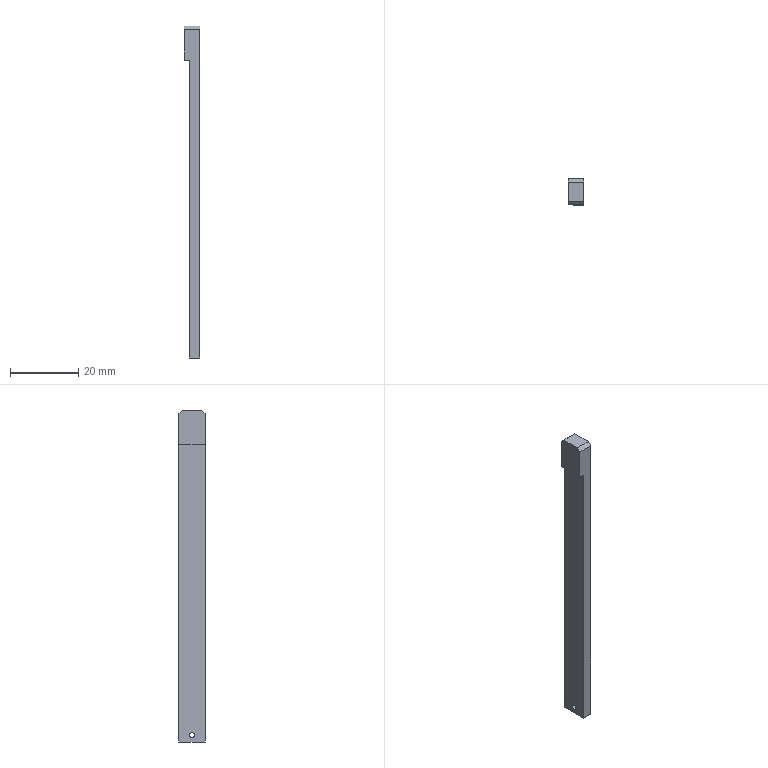Part | STEP file | slingshot detection spring block | 1 solid | 12 faces | box 4.5 x 7.6 x 97 mm | volume 2316 mm3 | plane 10 | cylinder 2 | commonest cylinder face diameters 1.5 x2
STEP:
#1=CARTESIAN_POINT('',(0.,0.,0.));
#2=DIRECTION('',(0.,0.,1.));
#3=DIRECTION('',(1.,0.,0.));
#4=AXIS2_PLACEMENT_3D('',#1,#2,#3);
#5=CARTESIAN_POINT('',(0.,-3.05,28.));
#6=VERTEX_POINT('',#5);
#7=CARTESIAN_POINT('',(3.,-3.05,28.));
#8=VERTEX_POINT('',#7);
#9=CARTESIAN_POINT('',(-22.,-3.05,28.));
#10=DIRECTION('',(1.,0.,0.));
#11=VECTOR('',#10,1.);
#12=LINE('',#9,#11);
#13=CARTESIAN_POINT('',(-22.,-3.8,28.));
#14=DIRECTION('',(1.,0.,0.));
#15=DIRECTION('',(0.,1.,0.));
#16=AXIS2_PLACEMENT_3D('',#13,#14,#15);
#17=CYLINDRICAL_SURFACE('',#16,0.75);
#18=CARTESIAN_POINT('',(6.283,0.));
#19=DIRECTION('',(0.,1.));
#20=VECTOR('',#19,1.);
#21=LINE('',#18,#20);
#22=(GEOMETRIC_REPRESENTATION_CONTEXT(2)PARAMETRIC_REPRESENTATION_CONTEXT()REPRESENTATION_CONTEXT('',''));
#23=DEFINITIONAL_REPRESENTATION('',(#21),#22);
#24=PCURVE('',#17,#23);
#25=CARTESIAN_POINT('',(-22.,-3.8,28.));
#26=DIRECTION('',(1.,0.,0.));
#27=DIRECTION('',(0.,1.,0.));
#28=AXIS2_PLACEMENT_3D('',#25,#26,#27);
#29=CYLINDRICAL_SURFACE('',#28,0.75);
#30=CARTESIAN_POINT('',(0.,0.));
#31=DIRECTION('',(0.,1.));
#32=VECTOR('',#31,1.);
#33=LINE('',#30,#32);
#34=(GEOMETRIC_REPRESENTATION_CONTEXT(2)PARAMETRIC_REPRESENTATION_CONTEXT()REPRESENTATION_CONTEXT('',''));
#35=DEFINITIONAL_REPRESENTATION('',(#33),#34);
#36=PCURVE('',#29,#35);
#37=SURFACE_CURVE('',#12,(#24,#36),.PCURVE_S1.);
#38=EDGE_CURVE('',#6,#8,#37,.T.);
#39=ORIENTED_EDGE('',*,*,#38,.T.);
#40=CARTESIAN_POINT('',(3.,-4.55,28.));
#41=VERTEX_POINT('',#40);
#42=CARTESIAN_POINT('',(3.,-3.8,28.));
#43=DIRECTION('',(1.,0.,0.));
#44=DIRECTION('',(0.,1.,0.));
#45=AXIS2_PLACEMENT_3D('',#42,#43,#44);
#46=CIRCLE('',#45,0.75);
#47=CARTESIAN_POINT('',(0.,25.));
#48=DIRECTION('',(1.,0.));
#49=VECTOR('',#48,1.);
#50=LINE('',#47,#49);
#51=(GEOMETRIC_REPRESENTATION_CONTEXT(2)PARAMETRIC_REPRESENTATION_CONTEXT()REPRESENTATION_CONTEXT('',''));
#52=DEFINITIONAL_REPRESENTATION('',(#50),#51);
#53=PCURVE('',#17,#52);
#54=CARTESIAN_POINT('',(3.,0.,123.));
#55=DIRECTION('',(-1.,0.,0.));
#56=DIRECTION('',(0.,-1.,0.));
#57=AXIS2_PLACEMENT_3D('',#54,#55,#56);
#58=PLANE('',#57);
#59=CARTESIAN_POINT('',(3.05,-95.));
#60=CARTESIAN_POINT('',(3.05,-93.701));
#61=CARTESIAN_POINT('',(4.175,-94.35));
#62=CARTESIAN_POINT('',(5.3,-95.));
#63=CARTESIAN_POINT('',(4.175,-95.65));
#64=CARTESIAN_POINT('',(3.05,-96.299));
#65=CARTESIAN_POINT('',(3.05,-95.));
#66=(BOUNDED_CURVE()B_SPLINE_CURVE(2,(#59,#60,#61,#62,#63,#64,#65),.UNSPECIFIED.,.T.,.F.)B_SPLINE_CURVE_WITH_KNOTS((1,2,2,2,2,1),(-2.094,0.,2.094,4.189,6.283,8.378),.UNSPECIFIED.)CURVE()GEOMETRIC_REPRESENTATION_ITEM()RATIONAL_B_SPLINE_CURVE((1.,0.5,1.,0.5,1.,0.5,1.))REPRESENTATION_ITEM(''));
#67=(GEOMETRIC_REPRESENTATION_CONTEXT(2)PARAMETRIC_REPRESENTATION_CONTEXT()REPRESENTATION_CONTEXT('',''));
#68=DEFINITIONAL_REPRESENTATION('',(#66),#67);
#69=PCURVE('',#58,#68);
#70=SURFACE_CURVE('',#46,(#53,#69),.PCURVE_S1.);
#71=EDGE_CURVE('',#41,#8,#70,.T.);
#72=ORIENTED_EDGE('',*,*,#71,.F.);
#73=CARTESIAN_POINT('',(0.,-4.55,28.));
#74=VERTEX_POINT('',#73);
#75=CARTESIAN_POINT('',(-22.,-4.55,28.));
#76=DIRECTION('',(1.,0.,0.));
#77=VECTOR('',#76,1.);
#78=LINE('',#75,#77);
#79=CARTESIAN_POINT('',(3.142,0.));
#80=DIRECTION('',(0.,1.));
#81=VECTOR('',#80,1.);
#82=LINE('',#79,#81);
#83=(GEOMETRIC_REPRESENTATION_CONTEXT(2)PARAMETRIC_REPRESENTATION_CONTEXT()REPRESENTATION_CONTEXT('',''));
#84=DEFINITIONAL_REPRESENTATION('',(#82),#83);
#85=PCURVE('',#17,#84);
#86=CARTESIAN_POINT('',(3.142,0.));
#87=DIRECTION('',(0.,1.));
#88=VECTOR('',#87,1.);
#89=LINE('',#86,#88);
#90=(GEOMETRIC_REPRESENTATION_CONTEXT(2)PARAMETRIC_REPRESENTATION_CONTEXT()REPRESENTATION_CONTEXT('',''));
#91=DEFINITIONAL_REPRESENTATION('',(#89),#90);
#92=PCURVE('',#29,#91);
#93=SURFACE_CURVE('',#78,(#85,#92),.PCURVE_S1.);
#94=EDGE_CURVE('',#74,#41,#93,.T.);
#95=ORIENTED_EDGE('',*,*,#94,.F.);
#96=CARTESIAN_POINT('',(0.,-3.8,28.));
#97=DIRECTION('',(1.,0.,0.));
#98=DIRECTION('',(0.,1.,0.));
#99=AXIS2_PLACEMENT_3D('',#96,#97,#98);
#100=CIRCLE('',#99,0.75);
#101=CARTESIAN_POINT('',(0.,22.));
#102=DIRECTION('',(1.,0.));
#103=VECTOR('',#102,1.);
#104=LINE('',#101,#103);
#105=(GEOMETRIC_REPRESENTATION_CONTEXT(2)PARAMETRIC_REPRESENTATION_CONTEXT()REPRESENTATION_CONTEXT('',''));
#106=DEFINITIONAL_REPRESENTATION('',(#104),#105);
#107=PCURVE('',#17,#106);
#108=CARTESIAN_POINT('',(0.,0.,123.));
#109=DIRECTION('',(1.,0.,0.));
#110=DIRECTION('',(0.,1.,0.));
#111=AXIS2_PLACEMENT_3D('',#108,#109,#110);
#112=PLANE('',#111);
#113=CARTESIAN_POINT('',(-3.8,-95.));
#114=DIRECTION('',(1.,0.));
#115=AXIS2_PLACEMENT_2D('',#113,#114);
#116=CIRCLE('',#115,0.75);
#117=(GEOMETRIC_REPRESENTATION_CONTEXT(2)PARAMETRIC_REPRESENTATION_CONTEXT()REPRESENTATION_CONTEXT('',''));
#118=DEFINITIONAL_REPRESENTATION('',(#116),#117);
#119=PCURVE('',#112,#118);
#120=SURFACE_CURVE('',#100,(#107,#119),.PCURVE_S1.);
#121=EDGE_CURVE('',#74,#6,#120,.T.);
#122=ORIENTED_EDGE('',*,*,#121,.T.);
#123=EDGE_LOOP('',(#39,#72,#95,#122));
#124=FACE_BOUND('',#123,.F.);
#125=ADVANCED_FACE('',(#124),#17,.F.);
#126=CARTESIAN_POINT('',(0.,-3.8,28.));
#127=DIRECTION('',(1.,0.,0.));
#128=DIRECTION('',(0.,1.,0.));
#129=AXIS2_PLACEMENT_3D('',#126,#127,#128);
#130=CIRCLE('',#129,0.75);
#131=CARTESIAN_POINT('',(-3.8,-95.));
#132=DIRECTION('',(1.,0.));
#133=AXIS2_PLACEMENT_2D('',#131,#132);
#134=CIRCLE('',#133,0.75);
#135=(GEOMETRIC_REPRESENTATION_CONTEXT(2)PARAMETRIC_REPRESENTATION_CONTEXT()REPRESENTATION_CONTEXT('',''));
#136=DEFINITIONAL_REPRESENTATION('',(#134),#135);
#137=PCURVE('',#112,#136);
#138=CARTESIAN_POINT('',(0.,22.));
#139=DIRECTION('',(1.,0.));
#140=VECTOR('',#139,1.);
#141=LINE('',#138,#140);
#142=(GEOMETRIC_REPRESENTATION_CONTEXT(2)PARAMETRIC_REPRESENTATION_CONTEXT()REPRESENTATION_CONTEXT('',''));
#143=DEFINITIONAL_REPRESENTATION('',(#141),#142);
#144=PCURVE('',#29,#143);
#145=SURFACE_CURVE('',#130,(#137,#144),.PCURVE_S1.);
#146=EDGE_CURVE('',#6,#74,#145,.T.);
#147=ORIENTED_EDGE('',*,*,#146,.T.);
#148=ORIENTED_EDGE('',*,*,#121,.T.);
#149=EDGE_LOOP('',(#147,#148));
#150=FACE_BOUND('',#149,.T.);
#151=CARTESIAN_POINT('',(0.,0.,113.));
#152=VERTEX_POINT('',#151);
#153=CARTESIAN_POINT('',(0.,-7.6,113.));
#154=VERTEX_POINT('',#153);
#155=CARTESIAN_POINT('',(0.,0.,113.));
#156=DIRECTION('',(0.,-1.,0.));
#157=VECTOR('',#156,1.);
#158=LINE('',#155,#157);
#159=CARTESIAN_POINT('',(0.,-10.));
#160=DIRECTION('',(-1.,0.));
#161=VECTOR('',#160,1.);
#162=LINE('',#159,#161);
#163=(GEOMETRIC_REPRESENTATION_CONTEXT(2)PARAMETRIC_REPRESENTATION_CONTEXT()REPRESENTATION_CONTEXT('',''));
#164=DEFINITIONAL_REPRESENTATION('',(#162),#163);
#165=PCURVE('',#112,#164);
#166=CARTESIAN_POINT('',(-1.5,0.,113.));
#167=DIRECTION('',(0.,0.,1.));
#168=DIRECTION('',(1.,0.,0.));
#169=AXIS2_PLACEMENT_3D('',#166,#167,#168);
#170=PLANE('',#169);
#171=CARTESIAN_POINT('',(1.5,0.));
#172=DIRECTION('',(0.,-1.));
#173=VECTOR('',#172,1.);
#174=LINE('',#171,#173);
#175=(GEOMETRIC_REPRESENTATION_CONTEXT(2)PARAMETRIC_REPRESENTATION_CONTEXT()REPRESENTATION_CONTEXT('',''));
#176=DEFINITIONAL_REPRESENTATION('',(#174),#175);
#177=PCURVE('',#170,#176);
#178=SURFACE_CURVE('',#158,(#165,#177),.PCURVE_S1.);
#179=EDGE_CURVE('',#152,#154,#178,.T.);
#180=ORIENTED_EDGE('',*,*,#179,.F.);
#181=CARTESIAN_POINT('',(0.,0.,26.));
#182=VERTEX_POINT('',#181);
#183=CARTESIAN_POINT('',(0.,0.,123.));
#184=DIRECTION('',(0.,0.,-1.));
#185=VECTOR('',#184,1.);
#186=LINE('',#183,#185);
#187=CARTESIAN_POINT('',(0.,0.));
#188=DIRECTION('',(0.,-1.));
#189=VECTOR('',#188,1.);
#190=LINE('',#187,#189);
#191=(GEOMETRIC_REPRESENTATION_CONTEXT(2)PARAMETRIC_REPRESENTATION_CONTEXT()REPRESENTATION_CONTEXT('',''));
#192=DEFINITIONAL_REPRESENTATION('',(#190),#191);
#193=PCURVE('',#112,#192);
#194=CARTESIAN_POINT('',(0.,0.,123.));
#195=DIRECTION('',(0.,-1.,0.));
#196=DIRECTION('',(0.,0.,-1.));
#197=AXIS2_PLACEMENT_3D('',#194,#195,#196);
#198=PLANE('',#197);
#199=CARTESIAN_POINT('',(0.,0.));
#200=DIRECTION('',(1.,0.));
#201=VECTOR('',#200,1.);
#202=LINE('',#199,#201);
#203=(GEOMETRIC_REPRESENTATION_CONTEXT(2)PARAMETRIC_REPRESENTATION_CONTEXT()REPRESENTATION_CONTEXT('',''));
#204=DEFINITIONAL_REPRESENTATION('',(#202),#203);
#205=PCURVE('',#198,#204);
#206=SURFACE_CURVE('',#186,(#193,#205),.PCURVE_S1.);
#207=EDGE_CURVE('',#152,#182,#206,.T.);
#208=ORIENTED_EDGE('',*,*,#207,.T.);
#209=CARTESIAN_POINT('',(0.,-7.6,26.));
#210=VERTEX_POINT('',#209);
#211=CARTESIAN_POINT('',(0.,16.05,26.));
#212=DIRECTION('',(0.,1.,0.));
#213=VECTOR('',#212,1.);
#214=LINE('',#211,#213);
#215=CARTESIAN_POINT('',(16.05,-97.));
#216=DIRECTION('',(1.,0.));
#217=VECTOR('',#216,1.);
#218=LINE('',#215,#217);
#219=(GEOMETRIC_REPRESENTATION_CONTEXT(2)PARAMETRIC_REPRESENTATION_CONTEXT()REPRESENTATION_CONTEXT('',''));
#220=DEFINITIONAL_REPRESENTATION('',(#218),#219);
#221=PCURVE('',#112,#220);
#222=CARTESIAN_POINT('',(10.,16.05,26.));
#223=DIRECTION('',(0.,0.,1.));
#224=DIRECTION('',(0.,-1.,0.));
#225=AXIS2_PLACEMENT_3D('',#222,#223,#224);
#226=PLANE('',#225);
#227=CARTESIAN_POINT('',(0.,-10.));
#228=DIRECTION('',(-1.,0.));
#229=VECTOR('',#228,1.);
#230=LINE('',#227,#229);
#231=(GEOMETRIC_REPRESENTATION_CONTEXT(2)PARAMETRIC_REPRESENTATION_CONTEXT()REPRESENTATION_CONTEXT('',''));
#232=DEFINITIONAL_REPRESENTATION('',(#230),#231);
#233=PCURVE('',#226,#232);
#234=SURFACE_CURVE('',#214,(#221,#233),.PCURVE_S1.);
#235=EDGE_CURVE('',#210,#182,#234,.T.);
#236=ORIENTED_EDGE('',*,*,#235,.F.);
#237=CARTESIAN_POINT('',(0.,-7.6,123.));
#238=DIRECTION('',(0.,0.,-1.));
#239=VECTOR('',#238,1.);
#240=LINE('',#237,#239);
#241=CARTESIAN_POINT('',(-7.6,0.));
#242=DIRECTION('',(0.,-1.));
#243=VECTOR('',#242,1.);
#244=LINE('',#241,#243);
#245=(GEOMETRIC_REPRESENTATION_CONTEXT(2)PARAMETRIC_REPRESENTATION_CONTEXT()REPRESENTATION_CONTEXT('',''));
#246=DEFINITIONAL_REPRESENTATION('',(#244),#245);
#247=PCURVE('',#112,#246);
#248=CARTESIAN_POINT('',(0.,-7.6,123.));
#249=DIRECTION('',(0.,1.,0.));
#250=DIRECTION('',(0.,0.,1.));
#251=AXIS2_PLACEMENT_3D('',#248,#249,#250);
#252=PLANE('',#251);
#253=CARTESIAN_POINT('',(0.,0.));
#254=DIRECTION('',(-1.,0.));
#255=VECTOR('',#254,1.);
#256=LINE('',#253,#255);
#257=(GEOMETRIC_REPRESENTATION_CONTEXT(2)PARAMETRIC_REPRESENTATION_CONTEXT()REPRESENTATION_CONTEXT('',''));
#258=DEFINITIONAL_REPRESENTATION('',(#256),#257);
#259=PCURVE('',#252,#258);
#260=SURFACE_CURVE('',#240,(#247,#259),.PCURVE_S1.);
#261=EDGE_CURVE('',#154,#210,#260,.T.);
#262=ORIENTED_EDGE('',*,*,#261,.F.);
#263=EDGE_LOOP('',(#180,#208,#236,#262));
#264=FACE_BOUND('',#263,.T.);
#265=ADVANCED_FACE('',(#150,#264),#112,.F.);
#266=CARTESIAN_POINT('',(3.,-7.6,122.));
#267=VERTEX_POINT('',#266);
#268=CARTESIAN_POINT('',(-1.5,-7.6,122.));
#269=VERTEX_POINT('',#268);
#270=CARTESIAN_POINT('',(0.,-7.6,122.));
#271=DIRECTION('',(-1.,0.,0.));
#272=VECTOR('',#271,1.);
#273=LINE('',#270,#272);
#274=CARTESIAN_POINT('',(-1.,0.));
#275=DIRECTION('',(0.,-1.));
#276=VECTOR('',#275,1.);
#277=LINE('',#274,#276);
#278=(GEOMETRIC_REPRESENTATION_CONTEXT(2)PARAMETRIC_REPRESENTATION_CONTEXT()REPRESENTATION_CONTEXT('',''));
#279=DEFINITIONAL_REPRESENTATION('',(#277),#278);
#280=PCURVE('',#252,#279);
#281=CARTESIAN_POINT('',(0.,-6.6,123.));
#282=DIRECTION('',(0.,-0.7071,0.7071));
#283=DIRECTION('',(0.,-0.7071,-0.7071));
#284=AXIS2_PLACEMENT_3D('',#281,#282,#283);
#285=PLANE('',#284);
#286=CARTESIAN_POINT('',(1.414,0.));
#287=DIRECTION('',(0.,-1.));
#288=VECTOR('',#287,1.);
#289=LINE('',#286,#288);
#290=(GEOMETRIC_REPRESENTATION_CONTEXT(2)PARAMETRIC_REPRESENTATION_CONTEXT()REPRESENTATION_CONTEXT('',''));
#291=DEFINITIONAL_REPRESENTATION('',(#289),#290);
#292=PCURVE('',#285,#291);
#293=SURFACE_CURVE('',#273,(#280,#292),.PCURVE_S1.);
#294=EDGE_CURVE('',#267,#269,#293,.T.);
#295=ORIENTED_EDGE('',*,*,#294,.T.);
#296=CARTESIAN_POINT('',(-1.5,-7.6,113.));
#297=VERTEX_POINT('',#296);
#298=CARTESIAN_POINT('',(-1.5,-7.6,113.));
#299=DIRECTION('',(0.,0.,1.));
#300=VECTOR('',#299,1.);
#301=LINE('',#298,#300);
#302=CARTESIAN_POINT('',(-10.,-1.5));
#303=DIRECTION('',(1.,0.));
#304=VECTOR('',#303,1.);
#305=LINE('',#302,#304);
#306=(GEOMETRIC_REPRESENTATION_CONTEXT(2)PARAMETRIC_REPRESENTATION_CONTEXT()REPRESENTATION_CONTEXT('',''));
#307=DEFINITIONAL_REPRESENTATION('',(#305),#306);
#308=PCURVE('',#252,#307);
#309=CARTESIAN_POINT('',(-1.5,-3.8,125.8));
#310=DIRECTION('',(1.,0.,0.));
#311=DIRECTION('',(0.,1.,0.));
#312=AXIS2_PLACEMENT_3D('',#309,#310,#311);
#313=PLANE('',#312);
#314=CARTESIAN_POINT('',(-3.8,-12.8));
#315=DIRECTION('',(0.,1.));
#316=VECTOR('',#315,1.);
#317=LINE('',#314,#316);
#318=(GEOMETRIC_REPRESENTATION_CONTEXT(2)PARAMETRIC_REPRESENTATION_CONTEXT()REPRESENTATION_CONTEXT('',''));
#319=DEFINITIONAL_REPRESENTATION('',(#317),#318);
#320=PCURVE('',#313,#319);
#321=SURFACE_CURVE('',#301,(#308,#320),.PCURVE_S1.);
#322=EDGE_CURVE('',#297,#269,#321,.T.);
#323=ORIENTED_EDGE('',*,*,#322,.F.);
#324=CARTESIAN_POINT('',(-1.5,-7.6,113.));
#325=DIRECTION('',(1.,0.,0.));
#326=VECTOR('',#325,1.);
#327=LINE('',#324,#326);
#328=CARTESIAN_POINT('',(-10.,-1.5));
#329=DIRECTION('',(0.,1.));
#330=VECTOR('',#329,1.);
#331=LINE('',#328,#330);
#332=(GEOMETRIC_REPRESENTATION_CONTEXT(2)PARAMETRIC_REPRESENTATION_CONTEXT()REPRESENTATION_CONTEXT('',''));
#333=DEFINITIONAL_REPRESENTATION('',(#331),#332);
#334=PCURVE('',#252,#333);
#335=CARTESIAN_POINT('',(0.,-7.6));
#336=DIRECTION('',(1.,0.));
#337=VECTOR('',#336,1.);
#338=LINE('',#335,#337);
#339=(GEOMETRIC_REPRESENTATION_CONTEXT(2)PARAMETRIC_REPRESENTATION_CONTEXT()REPRESENTATION_CONTEXT('',''));
#340=DEFINITIONAL_REPRESENTATION('',(#338),#339);
#341=PCURVE('',#170,#340);
#342=SURFACE_CURVE('',#327,(#334,#341),.PCURVE_S1.);
#343=EDGE_CURVE('',#297,#154,#342,.T.);
#344=ORIENTED_EDGE('',*,*,#343,.T.);
#345=ORIENTED_EDGE('',*,*,#261,.T.);
#346=CARTESIAN_POINT('',(3.,-7.6,26.));
#347=VERTEX_POINT('',#346);
#348=CARTESIAN_POINT('',(0.,-7.6,26.));
#349=DIRECTION('',(1.,0.,0.));
#350=VECTOR('',#349,1.);
#351=LINE('',#348,#350);
#352=CARTESIAN_POINT('',(-97.,0.));
#353=DIRECTION('',(0.,1.));
#354=VECTOR('',#353,1.);
#355=LINE('',#352,#354);
#356=(GEOMETRIC_REPRESENTATION_CONTEXT(2)PARAMETRIC_REPRESENTATION_CONTEXT()REPRESENTATION_CONTEXT('',''));
#357=DEFINITIONAL_REPRESENTATION('',(#355),#356);
#358=PCURVE('',#252,#357);
#359=CARTESIAN_POINT('',(23.65,-10.));
#360=DIRECTION('',(0.,1.));
#361=VECTOR('',#360,1.);
#362=LINE('',#359,#361);
#363=(GEOMETRIC_REPRESENTATION_CONTEXT(2)PARAMETRIC_REPRESENTATION_CONTEXT()REPRESENTATION_CONTEXT('',''));
#364=DEFINITIONAL_REPRESENTATION('',(#362),#363);
#365=PCURVE('',#226,#364);
#366=SURFACE_CURVE('',#351,(#358,#365),.PCURVE_S1.);
#367=EDGE_CURVE('',#210,#347,#366,.T.);
#368=ORIENTED_EDGE('',*,*,#367,.T.);
#369=CARTESIAN_POINT('',(3.,-7.6,123.));
#370=DIRECTION('',(0.,0.,-1.));
#371=VECTOR('',#370,1.);
#372=LINE('',#369,#371);
#373=CARTESIAN_POINT('',(0.,3.));
#374=DIRECTION('',(-1.,0.));
#375=VECTOR('',#374,1.);
#376=LINE('',#373,#375);
#377=(GEOMETRIC_REPRESENTATION_CONTEXT(2)PARAMETRIC_REPRESENTATION_CONTEXT()REPRESENTATION_CONTEXT('',''));
#378=DEFINITIONAL_REPRESENTATION('',(#376),#377);
#379=PCURVE('',#252,#378);
#380=CARTESIAN_POINT('',(7.6,0.));
#381=DIRECTION('',(0.,-1.));
#382=VECTOR('',#381,1.);
#383=LINE('',#380,#382);
#384=(GEOMETRIC_REPRESENTATION_CONTEXT(2)PARAMETRIC_REPRESENTATION_CONTEXT()REPRESENTATION_CONTEXT('',''));
#385=DEFINITIONAL_REPRESENTATION('',(#383),#384);
#386=PCURVE('',#58,#385);
#387=SURFACE_CURVE('',#372,(#379,#386),.PCURVE_S1.);
#388=EDGE_CURVE('',#267,#347,#387,.T.);
#389=ORIENTED_EDGE('',*,*,#388,.F.);
#390=EDGE_LOOP('',(#295,#323,#344,#345,#368,#389));
#391=FACE_BOUND('',#390,.T.);
#392=ADVANCED_FACE('',(#391),#252,.F.);
#393=CARTESIAN_POINT('',(3.,-3.8,28.));
#394=DIRECTION('',(1.,0.,0.));
#395=DIRECTION('',(0.,1.,0.));
#396=AXIS2_PLACEMENT_3D('',#393,#394,#395);
#397=CIRCLE('',#396,0.75);
#398=CARTESIAN_POINT('',(3.05,-95.));
#399=CARTESIAN_POINT('',(3.05,-93.701));
#400=CARTESIAN_POINT('',(4.175,-94.35));
#401=CARTESIAN_POINT('',(5.3,-95.));
#402=CARTESIAN_POINT('',(4.175,-95.65));
#403=CARTESIAN_POINT('',(3.05,-96.299));
#404=CARTESIAN_POINT('',(3.05,-95.));
#405=(BOUNDED_CURVE()B_SPLINE_CURVE(2,(#398,#399,#400,#401,#402,#403,#404),.UNSPECIFIED.,.T.,.F.)B_SPLINE_CURVE_WITH_KNOTS((1,2,2,2,2,1),(-2.094,0.,2.094,4.189,6.283,8.378),.UNSPECIFIED.)CURVE()GEOMETRIC_REPRESENTATION_ITEM()RATIONAL_B_SPLINE_CURVE((1.,0.5,1.,0.5,1.,0.5,1.))REPRESENTATION_ITEM(''));
#406=(GEOMETRIC_REPRESENTATION_CONTEXT(2)PARAMETRIC_REPRESENTATION_CONTEXT()REPRESENTATION_CONTEXT('',''));
#407=DEFINITIONAL_REPRESENTATION('',(#405),#406);
#408=PCURVE('',#58,#407);
#409=CARTESIAN_POINT('',(0.,25.));
#410=DIRECTION('',(1.,0.));
#411=VECTOR('',#410,1.);
#412=LINE('',#409,#411);
#413=(GEOMETRIC_REPRESENTATION_CONTEXT(2)PARAMETRIC_REPRESENTATION_CONTEXT()REPRESENTATION_CONTEXT('',''));
#414=DEFINITIONAL_REPRESENTATION('',(#412),#413);
#415=PCURVE('',#29,#414);
#416=SURFACE_CURVE('',#397,(#408,#415),.PCURVE_S1.);
#417=EDGE_CURVE('',#8,#41,#416,.T.);
#418=ORIENTED_EDGE('',*,*,#417,.F.);
#419=ORIENTED_EDGE('',*,*,#71,.F.);
#420=EDGE_LOOP('',(#418,#419));
#421=FACE_BOUND('',#420,.T.);
#422=ORIENTED_EDGE('',*,*,#388,.T.);
#423=CARTESIAN_POINT('',(3.,0.,26.));
#424=VERTEX_POINT('',#423);
#425=CARTESIAN_POINT('',(3.,0.,26.));
#426=DIRECTION('',(0.,1.,0.));
#427=VECTOR('',#426,1.);
#428=LINE('',#425,#427);
#429=CARTESIAN_POINT('',(0.,-97.));
#430=DIRECTION('',(-1.,0.));
#431=VECTOR('',#430,1.);
#432=LINE('',#429,#431);
#433=(GEOMETRIC_REPRESENTATION_CONTEXT(2)PARAMETRIC_REPRESENTATION_CONTEXT()REPRESENTATION_CONTEXT('',''));
#434=DEFINITIONAL_REPRESENTATION('',(#432),#433);
#435=PCURVE('',#58,#434);
#436=CARTESIAN_POINT('',(16.05,-7.));
#437=DIRECTION('',(-1.,0.));
#438=VECTOR('',#437,1.);
#439=LINE('',#436,#438);
#440=(GEOMETRIC_REPRESENTATION_CONTEXT(2)PARAMETRIC_REPRESENTATION_CONTEXT()REPRESENTATION_CONTEXT('',''));
#441=DEFINITIONAL_REPRESENTATION('',(#439),#440);
#442=PCURVE('',#226,#441);
#443=SURFACE_CURVE('',#428,(#435,#442),.PCURVE_S1.);
#444=EDGE_CURVE('',#347,#424,#443,.T.);
#445=ORIENTED_EDGE('',*,*,#444,.T.);
#446=CARTESIAN_POINT('',(3.,0.,122.));
#447=VERTEX_POINT('',#446);
#448=CARTESIAN_POINT('',(3.,0.,123.));
#449=DIRECTION('',(0.,0.,-1.));
#450=VECTOR('',#449,1.);
#451=LINE('',#448,#450);
#452=CARTESIAN_POINT('',(0.,0.));
#453=DIRECTION('',(0.,-1.));
#454=VECTOR('',#453,1.);
#455=LINE('',#452,#454);
#456=(GEOMETRIC_REPRESENTATION_CONTEXT(2)PARAMETRIC_REPRESENTATION_CONTEXT()REPRESENTATION_CONTEXT('',''));
#457=DEFINITIONAL_REPRESENTATION('',(#455),#456);
#458=PCURVE('',#58,#457);
#459=CARTESIAN_POINT('',(0.,3.));
#460=DIRECTION('',(1.,0.));
#461=VECTOR('',#460,1.);
#462=LINE('',#459,#461);
#463=(GEOMETRIC_REPRESENTATION_CONTEXT(2)PARAMETRIC_REPRESENTATION_CONTEXT()REPRESENTATION_CONTEXT('',''));
#464=DEFINITIONAL_REPRESENTATION('',(#462),#463);
#465=PCURVE('',#198,#464);
#466=SURFACE_CURVE('',#451,(#458,#465),.PCURVE_S1.);
#467=EDGE_CURVE('',#447,#424,#466,.T.);
#468=ORIENTED_EDGE('',*,*,#467,.F.);
#469=CARTESIAN_POINT('',(3.,-1.,123.));
#470=VERTEX_POINT('',#469);
#471=CARTESIAN_POINT('',(3.,-1.,123.));
#472=DIRECTION('',(0.,-0.7071,0.7071));
#473=VECTOR('',#472,1.);
#474=LINE('',#471,#473);
#475=CARTESIAN_POINT('',(1.,0.));
#476=DIRECTION('',(0.7071,0.7071));
#477=VECTOR('',#476,1.);
#478=LINE('',#475,#477);
#479=(GEOMETRIC_REPRESENTATION_CONTEXT(2)PARAMETRIC_REPRESENTATION_CONTEXT()REPRESENTATION_CONTEXT('',''));
#480=DEFINITIONAL_REPRESENTATION('',(#478),#479);
#481=PCURVE('',#58,#480);
#482=CARTESIAN_POINT('',(0.,-1.,123.));
#483=DIRECTION('',(0.,0.7071,0.7071));
#484=DIRECTION('',(0.,-0.7071,0.7071));
#485=AXIS2_PLACEMENT_3D('',#482,#483,#484);
#486=PLANE('',#485);
#487=CARTESIAN_POINT('',(0.,3.));
#488=DIRECTION('',(1.,0.));
#489=VECTOR('',#488,1.);
#490=LINE('',#487,#489);
#491=(GEOMETRIC_REPRESENTATION_CONTEXT(2)PARAMETRIC_REPRESENTATION_CONTEXT()REPRESENTATION_CONTEXT('',''));
#492=DEFINITIONAL_REPRESENTATION('',(#490),#491);
#493=PCURVE('',#486,#492);
#494=SURFACE_CURVE('',#474,(#481,#493),.PCURVE_S1.);
#495=EDGE_CURVE('',#447,#470,#494,.T.);
#496=ORIENTED_EDGE('',*,*,#495,.T.);
#497=CARTESIAN_POINT('',(3.,-6.6,123.));
#498=VERTEX_POINT('',#497);
#499=CARTESIAN_POINT('',(3.,0.,123.));
#500=DIRECTION('',(0.,1.,0.));
#501=VECTOR('',#500,1.);
#502=LINE('',#499,#501);
#503=CARTESIAN_POINT('',(0.,0.));
#504=DIRECTION('',(-1.,0.));
#505=VECTOR('',#504,1.);
#506=LINE('',#503,#505);
#507=(GEOMETRIC_REPRESENTATION_CONTEXT(2)PARAMETRIC_REPRESENTATION_CONTEXT()REPRESENTATION_CONTEXT('',''));
#508=DEFINITIONAL_REPRESENTATION('',(#506),#507);
#509=PCURVE('',#58,#508);
#510=CARTESIAN_POINT('',(0.,-7.6,123.));
#511=DIRECTION('',(0.,0.,1.));
#512=DIRECTION('',(1.,0.,0.));
#513=AXIS2_PLACEMENT_3D('',#510,#511,#512);
#514=PLANE('',#513);
#515=CARTESIAN_POINT('',(3.,7.6));
#516=DIRECTION('',(0.,1.));
#517=VECTOR('',#516,1.);
#518=LINE('',#515,#517);
#519=(GEOMETRIC_REPRESENTATION_CONTEXT(2)PARAMETRIC_REPRESENTATION_CONTEXT()REPRESENTATION_CONTEXT('',''));
#520=DEFINITIONAL_REPRESENTATION('',(#518),#519);
#521=PCURVE('',#514,#520);
#522=SURFACE_CURVE('',#502,(#509,#521),.PCURVE_S1.);
#523=EDGE_CURVE('',#498,#470,#522,.T.);
#524=ORIENTED_EDGE('',*,*,#523,.F.);
#525=CARTESIAN_POINT('',(3.,-6.6,123.));
#526=DIRECTION('',(0.,-0.7071,-0.7071));
#527=VECTOR('',#526,1.);
#528=LINE('',#525,#527);
#529=CARTESIAN_POINT('',(6.6,0.));
#530=DIRECTION('',(0.7071,-0.7071));
#531=VECTOR('',#530,1.);
#532=LINE('',#529,#531);
#533=(GEOMETRIC_REPRESENTATION_CONTEXT(2)PARAMETRIC_REPRESENTATION_CONTEXT()REPRESENTATION_CONTEXT('',''));
#534=DEFINITIONAL_REPRESENTATION('',(#532),#533);
#535=PCURVE('',#58,#534);
#536=CARTESIAN_POINT('',(0.,3.));
#537=DIRECTION('',(1.,0.));
#538=VECTOR('',#537,1.);
#539=LINE('',#536,#538);
#540=(GEOMETRIC_REPRESENTATION_CONTEXT(2)PARAMETRIC_REPRESENTATION_CONTEXT()REPRESENTATION_CONTEXT('',''));
#541=DEFINITIONAL_REPRESENTATION('',(#539),#540);
#542=PCURVE('',#285,#541);
#543=SURFACE_CURVE('',#528,(#535,#542),.PCURVE_S1.);
#544=EDGE_CURVE('',#498,#267,#543,.T.);
#545=ORIENTED_EDGE('',*,*,#544,.T.);
#546=EDGE_LOOP('',(#422,#445,#468,#496,#524,#545));
#547=FACE_BOUND('',#546,.T.);
#548=ADVANCED_FACE('',(#421,#547),#58,.F.);
#549=ORIENTED_EDGE('',*,*,#467,.T.);
#550=CARTESIAN_POINT('',(0.,0.,26.));
#551=DIRECTION('',(-1.,0.,0.));
#552=VECTOR('',#551,1.);
#553=LINE('',#550,#552);
#554=CARTESIAN_POINT('',(97.,0.));
#555=DIRECTION('',(0.,-1.));
#556=VECTOR('',#555,1.);
#557=LINE('',#554,#556);
#558=(GEOMETRIC_REPRESENTATION_CONTEXT(2)PARAMETRIC_REPRESENTATION_CONTEXT()REPRESENTATION_CONTEXT('',''));
#559=DEFINITIONAL_REPRESENTATION('',(#557),#558);
#560=PCURVE('',#198,#559);
#561=CARTESIAN_POINT('',(16.05,-10.));
#562=DIRECTION('',(0.,-1.));
#563=VECTOR('',#562,1.);
#564=LINE('',#561,#563);
#565=(GEOMETRIC_REPRESENTATION_CONTEXT(2)PARAMETRIC_REPRESENTATION_CONTEXT()REPRESENTATION_CONTEXT('',''));
#566=DEFINITIONAL_REPRESENTATION('',(#564),#565);
#567=PCURVE('',#226,#566);
#568=SURFACE_CURVE('',#553,(#560,#567),.PCURVE_S1.);
#569=EDGE_CURVE('',#424,#182,#568,.T.);
#570=ORIENTED_EDGE('',*,*,#569,.T.);
#571=ORIENTED_EDGE('',*,*,#207,.F.);
#572=CARTESIAN_POINT('',(-1.5,0.,113.));
#573=VERTEX_POINT('',#572);
#574=CARTESIAN_POINT('',(-1.5,0.,113.));
#575=DIRECTION('',(1.,0.,0.));
#576=VECTOR('',#575,1.);
#577=LINE('',#574,#576);
#578=CARTESIAN_POINT('',(10.,-1.5));
#579=DIRECTION('',(0.,1.));
#580=VECTOR('',#579,1.);
#581=LINE('',#578,#580);
#582=(GEOMETRIC_REPRESENTATION_CONTEXT(2)PARAMETRIC_REPRESENTATION_CONTEXT()REPRESENTATION_CONTEXT('',''));
#583=DEFINITIONAL_REPRESENTATION('',(#581),#582);
#584=PCURVE('',#198,#583);
#585=CARTESIAN_POINT('',(0.,0.));
#586=DIRECTION('',(1.,0.));
#587=VECTOR('',#586,1.);
#588=LINE('',#585,#587);
#589=(GEOMETRIC_REPRESENTATION_CONTEXT(2)PARAMETRIC_REPRESENTATION_CONTEXT()REPRESENTATION_CONTEXT('',''));
#590=DEFINITIONAL_REPRESENTATION('',(#588),#589);
#591=PCURVE('',#170,#590);
#592=SURFACE_CURVE('',#577,(#584,#591),.PCURVE_S1.);
#593=EDGE_CURVE('',#573,#152,#592,.T.);
#594=ORIENTED_EDGE('',*,*,#593,.F.);
#595=CARTESIAN_POINT('',(-1.5,0.,122.));
#596=VERTEX_POINT('',#595);
#597=CARTESIAN_POINT('',(-1.5,0.,122.));
#598=DIRECTION('',(0.,0.,-1.));
#599=VECTOR('',#598,1.);
#600=LINE('',#597,#599);
#601=CARTESIAN_POINT('',(1.,-1.5));
#602=DIRECTION('',(1.,0.));
#603=VECTOR('',#602,1.);
#604=LINE('',#601,#603);
#605=(GEOMETRIC_REPRESENTATION_CONTEXT(2)PARAMETRIC_REPRESENTATION_CONTEXT()REPRESENTATION_CONTEXT('',''));
#606=DEFINITIONAL_REPRESENTATION('',(#604),#605);
#607=PCURVE('',#198,#606);
#608=CARTESIAN_POINT('',(3.8,-3.8));
#609=DIRECTION('',(0.,-1.));
#610=VECTOR('',#609,1.);
#611=LINE('',#608,#610);
#612=(GEOMETRIC_REPRESENTATION_CONTEXT(2)PARAMETRIC_REPRESENTATION_CONTEXT()REPRESENTATION_CONTEXT('',''));
#613=DEFINITIONAL_REPRESENTATION('',(#611),#612);
#614=PCURVE('',#313,#613);
#615=SURFACE_CURVE('',#600,(#607,#614),.PCURVE_S1.);
#616=EDGE_CURVE('',#596,#573,#615,.T.);
#617=ORIENTED_EDGE('',*,*,#616,.F.);
#618=CARTESIAN_POINT('',(3.,0.,122.));
#619=DIRECTION('',(1.,0.,0.));
#620=VECTOR('',#619,1.);
#621=LINE('',#618,#620);
#622=CARTESIAN_POINT('',(1.,3.));
#623=DIRECTION('',(0.,1.));
#624=VECTOR('',#623,1.);
#625=LINE('',#622,#624);
#626=(GEOMETRIC_REPRESENTATION_CONTEXT(2)PARAMETRIC_REPRESENTATION_CONTEXT()REPRESENTATION_CONTEXT('',''));
#627=DEFINITIONAL_REPRESENTATION('',(#625),#626);
#628=PCURVE('',#198,#627);
#629=CARTESIAN_POINT('',(-1.414,3.));
#630=DIRECTION('',(0.,1.));
#631=VECTOR('',#630,1.);
#632=LINE('',#629,#631);
#633=(GEOMETRIC_REPRESENTATION_CONTEXT(2)PARAMETRIC_REPRESENTATION_CONTEXT()REPRESENTATION_CONTEXT('',''));
#634=DEFINITIONAL_REPRESENTATION('',(#632),#633);
#635=PCURVE('',#486,#634);
#636=SURFACE_CURVE('',#621,(#628,#635),.PCURVE_S1.);
#637=EDGE_CURVE('',#596,#447,#636,.T.);
#638=ORIENTED_EDGE('',*,*,#637,.T.);
#639=EDGE_LOOP('',(#549,#570,#571,#594,#617,#638));
#640=FACE_BOUND('',#639,.T.);
#641=ADVANCED_FACE('',(#640),#198,.F.);
#642=ORIENTED_EDGE('',*,*,#523,.T.);
#643=CARTESIAN_POINT('',(-1.5,-1.,123.));
#644=VERTEX_POINT('',#643);
#645=CARTESIAN_POINT('',(0.,-1.,123.));
#646=DIRECTION('',(-1.,0.,0.));
#647=VECTOR('',#646,1.);
#648=LINE('',#645,#647);
#649=CARTESIAN_POINT('',(0.,6.6));
#650=DIRECTION('',(-1.,0.));
#651=VECTOR('',#650,1.);
#652=LINE('',#649,#651);
#653=(GEOMETRIC_REPRESENTATION_CONTEXT(2)PARAMETRIC_REPRESENTATION_CONTEXT()REPRESENTATION_CONTEXT('',''));
#654=DEFINITIONAL_REPRESENTATION('',(#652),#653);
#655=PCURVE('',#514,#654);
#656=CARTESIAN_POINT('',(0.,0.));
#657=DIRECTION('',(0.,-1.));
#658=VECTOR('',#657,1.);
#659=LINE('',#656,#658);
#660=(GEOMETRIC_REPRESENTATION_CONTEXT(2)PARAMETRIC_REPRESENTATION_CONTEXT()REPRESENTATION_CONTEXT('',''));
#661=DEFINITIONAL_REPRESENTATION('',(#659),#660);
#662=PCURVE('',#486,#661);
#663=SURFACE_CURVE('',#648,(#655,#662),.PCURVE_S1.);
#664=EDGE_CURVE('',#470,#644,#663,.T.);
#665=ORIENTED_EDGE('',*,*,#664,.T.);
#666=CARTESIAN_POINT('',(-1.5,-6.6,123.));
#667=VERTEX_POINT('',#666);
#668=CARTESIAN_POINT('',(-1.5,-6.6,123.));
#669=DIRECTION('',(0.,1.,0.));
#670=VECTOR('',#669,1.);
#671=LINE('',#668,#670);
#672=CARTESIAN_POINT('',(-1.5,1.));
#673=DIRECTION('',(0.,1.));
#674=VECTOR('',#673,1.);
#675=LINE('',#672,#674);
#676=(GEOMETRIC_REPRESENTATION_CONTEXT(2)PARAMETRIC_REPRESENTATION_CONTEXT()REPRESENTATION_CONTEXT('',''));
#677=DEFINITIONAL_REPRESENTATION('',(#675),#676);
#678=PCURVE('',#514,#677);
#679=CARTESIAN_POINT('',(-2.8,-2.8));
#680=DIRECTION('',(1.,0.));
#681=VECTOR('',#680,1.);
#682=LINE('',#679,#681);
#683=(GEOMETRIC_REPRESENTATION_CONTEXT(2)PARAMETRIC_REPRESENTATION_CONTEXT()REPRESENTATION_CONTEXT('',''));
#684=DEFINITIONAL_REPRESENTATION('',(#682),#683);
#685=PCURVE('',#313,#684);
#686=SURFACE_CURVE('',#671,(#678,#685),.PCURVE_S1.);
#687=EDGE_CURVE('',#667,#644,#686,.T.);
#688=ORIENTED_EDGE('',*,*,#687,.F.);
#689=CARTESIAN_POINT('',(3.,-6.6,123.));
#690=DIRECTION('',(1.,0.,0.));
#691=VECTOR('',#690,1.);
#692=LINE('',#689,#691);
#693=CARTESIAN_POINT('',(3.,1.));
#694=DIRECTION('',(1.,0.));
#695=VECTOR('',#694,1.);
#696=LINE('',#693,#695);
#697=(GEOMETRIC_REPRESENTATION_CONTEXT(2)PARAMETRIC_REPRESENTATION_CONTEXT()REPRESENTATION_CONTEXT('',''));
#698=DEFINITIONAL_REPRESENTATION('',(#696),#697);
#699=PCURVE('',#514,#698);
#700=CARTESIAN_POINT('',(0.,3.));
#701=DIRECTION('',(0.,1.));
#702=VECTOR('',#701,1.);
#703=LINE('',#700,#702);
#704=(GEOMETRIC_REPRESENTATION_CONTEXT(2)PARAMETRIC_REPRESENTATION_CONTEXT()REPRESENTATION_CONTEXT('',''));
#705=DEFINITIONAL_REPRESENTATION('',(#703),#704);
#706=PCURVE('',#285,#705);
#707=SURFACE_CURVE('',#692,(#699,#706),.PCURVE_S1.);
#708=EDGE_CURVE('',#667,#498,#707,.T.);
#709=ORIENTED_EDGE('',*,*,#708,.T.);
#710=EDGE_LOOP('',(#642,#665,#688,#709));
#711=FACE_BOUND('',#710,.T.);
#712=ADVANCED_FACE('',(#711),#514,.T.);
#713=ORIENTED_EDGE('',*,*,#495,.F.);
#714=ORIENTED_EDGE('',*,*,#637,.F.);
#715=CARTESIAN_POINT('',(-1.5,-1.,123.));
#716=DIRECTION('',(0.,0.7071,-0.7071));
#717=VECTOR('',#716,1.);
#718=LINE('',#715,#717);
#719=CARTESIAN_POINT('',(0.,-1.5));
#720=DIRECTION('',(-1.,0.));
#721=VECTOR('',#720,1.);
#722=LINE('',#719,#721);
#723=(GEOMETRIC_REPRESENTATION_CONTEXT(2)PARAMETRIC_REPRESENTATION_CONTEXT()REPRESENTATION_CONTEXT('',''));
#724=DEFINITIONAL_REPRESENTATION('',(#722),#723);
#725=PCURVE('',#486,#724);
#726=CARTESIAN_POINT('',(2.8,-2.8));
#727=DIRECTION('',(0.7071,-0.7071));
#728=VECTOR('',#727,1.);
#729=LINE('',#726,#728);
#730=(GEOMETRIC_REPRESENTATION_CONTEXT(2)PARAMETRIC_REPRESENTATION_CONTEXT()REPRESENTATION_CONTEXT('',''));
#731=DEFINITIONAL_REPRESENTATION('',(#729),#730);
#732=PCURVE('',#313,#731);
#733=SURFACE_CURVE('',#718,(#725,#732),.PCURVE_S1.);
#734=EDGE_CURVE('',#644,#596,#733,.T.);
#735=ORIENTED_EDGE('',*,*,#734,.F.);
#736=ORIENTED_EDGE('',*,*,#664,.F.);
#737=EDGE_LOOP('',(#713,#714,#735,#736));
#738=FACE_BOUND('',#737,.T.);
#739=ADVANCED_FACE('',(#738),#486,.T.);
#740=ORIENTED_EDGE('',*,*,#708,.F.);
#741=CARTESIAN_POINT('',(-1.5,-7.6,122.));
#742=DIRECTION('',(0.,0.7071,0.7071));
#743=VECTOR('',#742,1.);
#744=LINE('',#741,#743);
#745=CARTESIAN_POINT('',(1.414,-1.5));
#746=DIRECTION('',(-1.,0.));
#747=VECTOR('',#746,1.);
#748=LINE('',#745,#747);
#749=(GEOMETRIC_REPRESENTATION_CONTEXT(2)PARAMETRIC_REPRESENTATION_CONTEXT()REPRESENTATION_CONTEXT('',''));
#750=DEFINITIONAL_REPRESENTATION('',(#748),#749);
#751=PCURVE('',#285,#750);
#752=CARTESIAN_POINT('',(-3.8,-3.8));
#753=DIRECTION('',(0.7071,0.7071));
#754=VECTOR('',#753,1.);
#755=LINE('',#752,#754);
#756=(GEOMETRIC_REPRESENTATION_CONTEXT(2)PARAMETRIC_REPRESENTATION_CONTEXT()REPRESENTATION_CONTEXT('',''));
#757=DEFINITIONAL_REPRESENTATION('',(#755),#756);
#758=PCURVE('',#313,#757);
#759=SURFACE_CURVE('',#744,(#751,#758),.PCURVE_S1.);
#760=EDGE_CURVE('',#269,#667,#759,.T.);
#761=ORIENTED_EDGE('',*,*,#760,.F.);
#762=ORIENTED_EDGE('',*,*,#294,.F.);
#763=ORIENTED_EDGE('',*,*,#544,.F.);
#764=EDGE_LOOP('',(#740,#761,#762,#763));
#765=FACE_BOUND('',#764,.T.);
#766=ADVANCED_FACE('',(#765),#285,.T.);
#767=ORIENTED_EDGE('',*,*,#417,.F.);
#768=ORIENTED_EDGE('',*,*,#38,.F.);
#769=ORIENTED_EDGE('',*,*,#146,.T.);
#770=ORIENTED_EDGE('',*,*,#94,.T.);
#771=EDGE_LOOP('',(#767,#768,#769,#770));
#772=FACE_BOUND('',#771,.F.);
#773=ADVANCED_FACE('',(#772),#29,.F.);
#774=ORIENTED_EDGE('',*,*,#235,.T.);
#775=ORIENTED_EDGE('',*,*,#569,.F.);
#776=ORIENTED_EDGE('',*,*,#444,.F.);
#777=ORIENTED_EDGE('',*,*,#367,.F.);
#778=EDGE_LOOP('',(#774,#775,#776,#777));
#779=FACE_BOUND('',#778,.T.);
#780=ADVANCED_FACE('',(#779),#226,.F.);
#781=ORIENTED_EDGE('',*,*,#179,.T.);
#782=ORIENTED_EDGE('',*,*,#343,.F.);
#783=CARTESIAN_POINT('',(-1.5,0.,113.));
#784=DIRECTION('',(0.,-1.,0.));
#785=VECTOR('',#784,1.);
#786=LINE('',#783,#785);
#787=CARTESIAN_POINT('',(0.,0.));
#788=DIRECTION('',(0.,-1.));
#789=VECTOR('',#788,1.);
#790=LINE('',#787,#789);
#791=(GEOMETRIC_REPRESENTATION_CONTEXT(2)PARAMETRIC_REPRESENTATION_CONTEXT()REPRESENTATION_CONTEXT('',''));
#792=DEFINITIONAL_REPRESENTATION('',(#790),#791);
#793=PCURVE('',#170,#792);
#794=CARTESIAN_POINT('',(3.8,-12.8));
#795=DIRECTION('',(-1.,0.));
#796=VECTOR('',#795,1.);
#797=LINE('',#794,#796);
#798=(GEOMETRIC_REPRESENTATION_CONTEXT(2)PARAMETRIC_REPRESENTATION_CONTEXT()REPRESENTATION_CONTEXT('',''));
#799=DEFINITIONAL_REPRESENTATION('',(#797),#798);
#800=PCURVE('',#313,#799);
#801=SURFACE_CURVE('',#786,(#793,#800),.PCURVE_S1.);
#802=EDGE_CURVE('',#573,#297,#801,.T.);
#803=ORIENTED_EDGE('',*,*,#802,.F.);
#804=ORIENTED_EDGE('',*,*,#593,.T.);
#805=EDGE_LOOP('',(#781,#782,#803,#804));
#806=FACE_BOUND('',#805,.T.);
#807=ADVANCED_FACE('',(#806),#170,.F.);
#808=ORIENTED_EDGE('',*,*,#734,.T.);
#809=ORIENTED_EDGE('',*,*,#616,.T.);
#810=ORIENTED_EDGE('',*,*,#802,.T.);
#811=ORIENTED_EDGE('',*,*,#322,.T.);
#812=ORIENTED_EDGE('',*,*,#760,.T.);
#813=ORIENTED_EDGE('',*,*,#687,.T.);
#814=EDGE_LOOP('',(#808,#809,#810,#811,#812,#813));
#815=FACE_BOUND('',#814,.T.);
#816=ADVANCED_FACE('',(#815),#313,.F.);
#817=CLOSED_SHELL('',(#125,#265,#392,#548,#641,#712,#739,#766,#773,#780,#807,#816));
#818=MANIFOLD_SOLID_BREP('',#817);
#819=(LENGTH_UNIT()NAMED_UNIT(*)SI_UNIT(.MILLI.,.METRE.));
#820=UNCERTAINTY_MEASURE_WITH_UNIT(LENGTH_MEASURE(0.0000001),#819,'','');
#821=(NAMED_UNIT(*)PLANE_ANGLE_UNIT()SI_UNIT($,.RADIAN.));
#822=(NAMED_UNIT(*)SI_UNIT($,.STERADIAN.)SOLID_ANGLE_UNIT());
#823=(GEOMETRIC_REPRESENTATION_CONTEXT(3)GLOBAL_UNCERTAINTY_ASSIGNED_CONTEXT((#820))GLOBAL_UNIT_ASSIGNED_CONTEXT((#819,#821,#822))REPRESENTATION_CONTEXT('',''));
#824=ADVANCED_BREP_SHAPE_REPRESENTATION('',(#4,#818),#823);